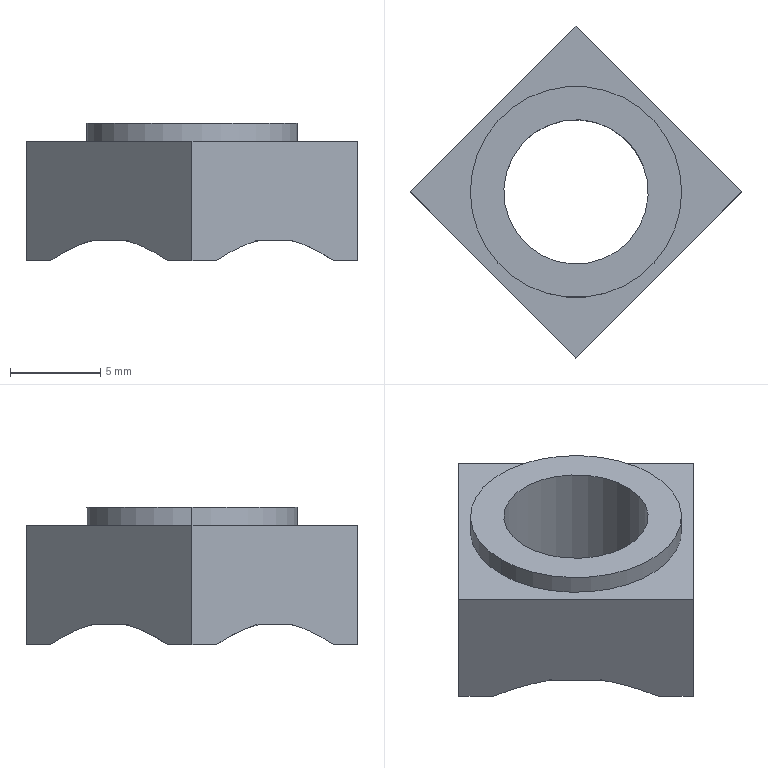Part | STEP file | Q37108 | 1 solid | 20 faces | box 18.385 x 18.385 x 7.6 mm | volume 729.18 mm3 | plane 11 | cone 5 | cylinder 4 | commonest cylinder face diameters 8 x2 11.7 x2
STEP:
#1=CARTESIAN_POINT('',(3.672,5.52,0.));
#2=VERTEX_POINT('',#1);
#3=CARTESIAN_POINT('',(5.52,3.672,0.));
#4=VERTEX_POINT('',#3);
#5=CARTESIAN_POINT('',(4.596,4.596,0.));
#6=DIRECTION('',(0.7071,-0.7071,0.));
#7=VECTOR('',#6,1.);
#8=LINE('',#5,#7);
#9=EDGE_CURVE('',#2,#4,#8,.T.);
#10=ORIENTED_EDGE('',*,*,#9,.T.);
#11=CARTESIAN_POINT('',(5.818,3.179,0.));
#12=VERTEX_POINT('',#11);
#13=CARTESIAN_POINT('',(0.,0.,0.));
#14=DIRECTION('',(0.,0.,1.));
#15=AXIS2_PLACEMENT_3D('',#13,#14,$);
#16=CIRCLE('',#15,6.63);
#17=EDGE_CURVE('',#12,#4,#16,.T.);
#18=ORIENTED_EDGE('',*,*,#17,.F.);
#19=CARTESIAN_POINT('',(5.52,-3.672,0.));
#20=VERTEX_POINT('',#19);
#21=CARTESIAN_POINT('',(0.,0.,0.));
#22=DIRECTION('',(0.,0.,1.));
#23=AXIS2_PLACEMENT_3D('',#21,#22,$);
#24=CIRCLE('',#23,6.63);
#25=EDGE_CURVE('',#20,#12,#24,.T.);
#26=ORIENTED_EDGE('',*,*,#25,.F.);
#27=CARTESIAN_POINT('',(3.672,-5.52,0.));
#28=VERTEX_POINT('',#27);
#29=CARTESIAN_POINT('',(4.596,-4.596,0.));
#30=DIRECTION('',(-0.7071,-0.7071,0.));
#31=VECTOR('',#30,1.);
#32=LINE('',#29,#31);
#33=EDGE_CURVE('',#20,#28,#32,.T.);
#34=ORIENTED_EDGE('',*,*,#33,.T.);
#35=CARTESIAN_POINT('',(-3.672,-5.52,0.));
#36=VERTEX_POINT('',#35);
#37=CARTESIAN_POINT('',(0.,0.,0.));
#38=DIRECTION('',(0.,0.,1.));
#39=AXIS2_PLACEMENT_3D('',#37,#38,$);
#40=CIRCLE('',#39,6.63);
#41=EDGE_CURVE('',#36,#28,#40,.T.);
#42=ORIENTED_EDGE('',*,*,#41,.F.);
#43=CARTESIAN_POINT('',(-5.52,-3.672,0.));
#44=VERTEX_POINT('',#43);
#45=CARTESIAN_POINT('',(-4.596,-4.596,0.));
#46=DIRECTION('',(0.7071,-0.7071,0.));
#47=VECTOR('',#46,1.);
#48=LINE('',#45,#47);
#49=EDGE_CURVE('',#44,#36,#48,.T.);
#50=ORIENTED_EDGE('',*,*,#49,.F.);
#51=CARTESIAN_POINT('',(-5.818,-3.179,0.));
#52=VERTEX_POINT('',#51);
#53=CARTESIAN_POINT('',(0.,0.,0.));
#54=DIRECTION('',(0.,0.,1.));
#55=AXIS2_PLACEMENT_3D('',#53,#54,$);
#56=CIRCLE('',#55,6.63);
#57=EDGE_CURVE('',#52,#44,#56,.T.);
#58=ORIENTED_EDGE('',*,*,#57,.F.);
#59=CARTESIAN_POINT('',(-5.52,3.672,0.));
#60=VERTEX_POINT('',#59);
#61=CARTESIAN_POINT('',(0.,0.,0.));
#62=DIRECTION('',(0.,0.,1.));
#63=AXIS2_PLACEMENT_3D('',#61,#62,$);
#64=CIRCLE('',#63,6.63);
#65=EDGE_CURVE('',#60,#52,#64,.T.);
#66=ORIENTED_EDGE('',*,*,#65,.F.);
#67=CARTESIAN_POINT('',(-3.672,5.52,0.));
#68=VERTEX_POINT('',#67);
#69=CARTESIAN_POINT('',(-4.596,4.596,0.));
#70=DIRECTION('',(0.7071,0.7071,0.));
#71=VECTOR('',#70,1.);
#72=LINE('',#69,#71);
#73=EDGE_CURVE('',#60,#68,#72,.T.);
#74=ORIENTED_EDGE('',*,*,#73,.T.);
#75=CARTESIAN_POINT('',(0.,0.,0.));
#76=DIRECTION('',(0.,0.,1.));
#77=AXIS2_PLACEMENT_3D('',#75,#76,$);
#78=CIRCLE('',#77,6.63);
#79=EDGE_CURVE('',#2,#68,#78,.T.);
#80=ORIENTED_EDGE('',*,*,#79,.F.);
#81=EDGE_LOOP('',(#10,#18,#26,#34,#42,#50,#58,#66,#74,#80));
#82=FACE_OUTER_BOUND('',#81,.T.);
#83=CARTESIAN_POINT('',(-3.51,1.918,0.));
#84=VERTEX_POINT('',#83);
#85=CARTESIAN_POINT('',(3.51,-1.918,0.));
#86=VERTEX_POINT('',#85);
#87=CARTESIAN_POINT('',(0.,0.,0.));
#88=DIRECTION('',(0.,0.,1.));
#89=AXIS2_PLACEMENT_3D('',#87,#88,$);
#90=CIRCLE('',#89,4.);
#91=EDGE_CURVE('',#84,#86,#90,.T.);
#92=ORIENTED_EDGE('',*,*,#91,.T.);
#93=CARTESIAN_POINT('',(0.,0.,0.));
#94=DIRECTION('',(0.,0.,1.));
#95=AXIS2_PLACEMENT_3D('',#93,#94,$);
#96=CIRCLE('',#95,4.);
#97=EDGE_CURVE('',#86,#84,#96,.T.);
#98=ORIENTED_EDGE('',*,*,#97,.T.);
#99=EDGE_LOOP('',(#92,#98));
#100=FACE_BOUND('',#99,.T.);
#101=CARTESIAN_POINT('',(0.,0.,0.));
#102=DIRECTION('',(0.,0.,1.));
#103=DIRECTION('',(1.,0.,0.));
#104=AXIS2_PLACEMENT_3D('',#101,#102,#103);
#105=PLANE('',#104);
#106=ADVANCED_FACE('',(#82,#100),#105,.F.);
#107=CARTESIAN_POINT('',(-1.371,7.822,-1.1));
#108=VERTEX_POINT('',#107);
#109=CARTESIAN_POINT('',(-3.672,5.52,0.));
#110=CARTESIAN_POINT('',(-3.177,6.016,-0.1159));
#111=CARTESIAN_POINT('',(-2.653,6.539,-0.3192));
#112=CARTESIAN_POINT('',(-2.077,7.115,-0.6183));
#113=CARTESIAN_POINT('',(-1.371,7.822,-1.1));
#114=B_SPLINE_CURVE_WITH_KNOTS('',4,(#109,#110,#111,#112,#113),.UNSPECIFIED.,.F.,.U.,(5,5),(0.,41.553),.UNSPECIFIED.);
#115=EDGE_CURVE('',#68,#108,#114,.T.);
#116=ORIENTED_EDGE('',*,*,#115,.T.);
#117=CARTESIAN_POINT('',(1.371,7.822,-1.1));
#118=VERTEX_POINT('',#117);
#119=CARTESIAN_POINT('',(0.,0.,-1.1));
#120=DIRECTION('',(0.,0.,-1.));
#121=AXIS2_PLACEMENT_3D('',#119,#120,$);
#122=CIRCLE('',#121,7.941);
#123=EDGE_CURVE('',#118,#108,#122,.F.);
#124=ORIENTED_EDGE('',*,*,#123,.F.);
#125=CARTESIAN_POINT('',(3.672,5.52,0.));
#126=CARTESIAN_POINT('',(3.177,6.016,-0.1159));
#127=CARTESIAN_POINT('',(2.653,6.539,-0.3192));
#128=CARTESIAN_POINT('',(2.077,7.115,-0.6183));
#129=CARTESIAN_POINT('',(1.371,7.822,-1.1));
#130=B_SPLINE_CURVE_WITH_KNOTS('',4,(#125,#126,#127,#128,#129),.UNSPECIFIED.,.F.,.U.,(5,5),(0.,41.553),.UNSPECIFIED.);
#131=EDGE_CURVE('',#2,#118,#130,.T.);
#132=ORIENTED_EDGE('',*,*,#131,.F.);
#133=ORIENTED_EDGE('',*,*,#79,.T.);
#134=EDGE_LOOP('',(#116,#124,#132,#133));
#135=FACE_OUTER_BOUND('',#134,.T.);
#136=CARTESIAN_POINT('',(0.,0.,0.));
#137=DIRECTION('',(0.,0.,-1.));
#138=DIRECTION('',(0.8776,0.4794,0.));
#139=AXIS2_PLACEMENT_3D('',#136,#137,#138);
#140=CONICAL_SURFACE('',#139,6.63,0.8727);
#141=ADVANCED_FACE('',(#135),#140,.F.);
#142=ORIENTED_EDGE('',*,*,#115,.F.);
#143=ORIENTED_EDGE('',*,*,#73,.F.);
#144=CARTESIAN_POINT('',(-7.822,1.371,-1.1));
#145=VERTEX_POINT('',#144);
#146=CARTESIAN_POINT('',(-5.52,3.672,0.));
#147=CARTESIAN_POINT('',(-5.821,3.371,-0.0704));
#148=CARTESIAN_POINT('',(-6.132,3.061,-0.1706));
#149=CARTESIAN_POINT('',(-6.456,2.736,-0.3034));
#150=CARTESIAN_POINT('',(-6.913,2.279,-0.5286));
#151=CARTESIAN_POINT('',(-7.427,1.765,-0.8406));
#152=CARTESIAN_POINT('',(-7.554,1.638,-0.921));
#153=CARTESIAN_POINT('',(-7.686,1.507,-1.007));
#154=CARTESIAN_POINT('',(-7.822,1.371,-1.1));
#155=B_SPLINE_CURVE_WITH_KNOTS('',5,(#146,#147,#148,#149,#150,#151,#152,#153,#154),.UNSPECIFIED.,.F.,.U.,(6,3,6),(0.,31.556,41.553),.UNSPECIFIED.);
#156=EDGE_CURVE('',#60,#145,#155,.T.);
#157=ORIENTED_EDGE('',*,*,#156,.T.);
#158=CARTESIAN_POINT('',(-9.192,0.,-1.1));
#159=VERTEX_POINT('',#158);
#160=CARTESIAN_POINT('',(-8.507,0.6853,-1.1));
#161=DIRECTION('',(0.7071,0.7071,0.));
#162=VECTOR('',#161,1.);
#163=LINE('',#160,#162);
#164=EDGE_CURVE('',#145,#159,#163,.F.);
#165=ORIENTED_EDGE('',*,*,#164,.T.);
#166=CARTESIAN_POINT('',(-9.192,0.,5.5));
#167=VERTEX_POINT('',#166);
#168=CARTESIAN_POINT('',(-9.192,0.,2.2));
#169=DIRECTION('',(0.,0.,1.));
#170=VECTOR('',#169,1.);
#171=LINE('',#168,#170);
#172=EDGE_CURVE('',#159,#167,#171,.T.);
#173=ORIENTED_EDGE('',*,*,#172,.T.);
#174=CARTESIAN_POINT('',(0.,9.192,5.5));
#175=VERTEX_POINT('',#174);
#176=CARTESIAN_POINT('',(-4.596,4.596,5.5));
#177=DIRECTION('',(0.7071,0.7071,0.));
#178=VECTOR('',#177,1.);
#179=LINE('',#176,#178);
#180=EDGE_CURVE('',#175,#167,#179,.F.);
#181=ORIENTED_EDGE('',*,*,#180,.F.);
#182=CARTESIAN_POINT('',(0.,9.192,-1.1));
#183=VERTEX_POINT('',#182);
#184=CARTESIAN_POINT('',(0.,9.192,2.2));
#185=DIRECTION('',(0.,0.,1.));
#186=VECTOR('',#185,1.);
#187=LINE('',#184,#186);
#188=EDGE_CURVE('',#183,#175,#187,.T.);
#189=ORIENTED_EDGE('',*,*,#188,.F.);
#190=CARTESIAN_POINT('',(-0.6853,8.507,-1.1));
#191=DIRECTION('',(0.7071,0.7071,0.));
#192=VECTOR('',#191,1.);
#193=LINE('',#190,#192);
#194=EDGE_CURVE('',#183,#108,#193,.F.);
#195=ORIENTED_EDGE('',*,*,#194,.T.);
#196=EDGE_LOOP('',(#142,#143,#157,#165,#173,#181,#189,#195));
#197=FACE_OUTER_BOUND('',#196,.T.);
#198=CARTESIAN_POINT('',(-9.192,0.,0.));
#199=DIRECTION('',(0.7071,-0.7071,0.));
#200=DIRECTION('',(0.7071,0.7071,0.));
#201=AXIS2_PLACEMENT_3D('',#198,#199,#200);
#202=PLANE('',#201);
#203=ADVANCED_FACE('',(#197),#202,.F.);
#204=CARTESIAN_POINT('',(-5.945,-3.248,-0.1208));
#205=VERTEX_POINT('',#204);
#206=CARTESIAN_POINT('',(-5.52,-3.672,0.));
#207=CARTESIAN_POINT('',(-5.659,-3.534,-0.03245));
#208=CARTESIAN_POINT('',(-5.8,-3.392,-0.07246));
#209=CARTESIAN_POINT('',(-5.945,-3.248,-0.1208));
#210=B_SPLINE_CURVE_WITH_KNOTS('',3,(#206,#207,#208,#209),.UNSPECIFIED.,.F.,.U.,(4,4),(0.,8.728),.UNSPECIFIED.);
#211=EDGE_CURVE('',#44,#205,#210,.T.);
#212=ORIENTED_EDGE('',*,*,#211,.T.);
#213=CARTESIAN_POINT('',(-7.822,-1.371,-1.1));
#214=VERTEX_POINT('',#213);
#215=CARTESIAN_POINT('',(-5.945,-3.248,-0.1208));
#216=CARTESIAN_POINT('',(-6.353,-2.839,-0.2573));
#217=CARTESIAN_POINT('',(-6.788,-2.405,-0.4537));
#218=CARTESIAN_POINT('',(-7.263,-1.929,-0.7194));
#219=CARTESIAN_POINT('',(-7.822,-1.371,-1.1));
#220=B_SPLINE_CURVE_WITH_KNOTS('',4,(#215,#216,#217,#218,#219),.UNSPECIFIED.,.F.,.U.,(5,5),(0.,32.828),.UNSPECIFIED.);
#221=EDGE_CURVE('',#205,#214,#220,.T.);
#222=ORIENTED_EDGE('',*,*,#221,.T.);
#223=CARTESIAN_POINT('',(0.,0.,-1.1));
#224=DIRECTION('',(0.,0.,-1.));
#225=AXIS2_PLACEMENT_3D('',#223,#224,$);
#226=CIRCLE('',#225,7.941);
#227=EDGE_CURVE('',#145,#214,#226,.F.);
#228=ORIENTED_EDGE('',*,*,#227,.F.);
#229=ORIENTED_EDGE('',*,*,#156,.F.);
#230=ORIENTED_EDGE('',*,*,#65,.T.);
#231=ORIENTED_EDGE('',*,*,#57,.T.);
#232=EDGE_LOOP('',(#212,#222,#228,#229,#230,#231));
#233=FACE_OUTER_BOUND('',#232,.T.);
#234=ADVANCED_FACE('',(#233),#140,.F.);
#235=ORIENTED_EDGE('',*,*,#221,.F.);
#236=ORIENTED_EDGE('',*,*,#211,.F.);
#237=ORIENTED_EDGE('',*,*,#49,.T.);
#238=CARTESIAN_POINT('',(-1.371,-7.822,-1.1));
#239=VERTEX_POINT('',#238);
#240=CARTESIAN_POINT('',(-3.672,-5.52,0.));
#241=CARTESIAN_POINT('',(-3.371,-5.821,-0.0704));
#242=CARTESIAN_POINT('',(-3.061,-6.132,-0.1706));
#243=CARTESIAN_POINT('',(-2.736,-6.456,-0.3034));
#244=CARTESIAN_POINT('',(-2.279,-6.913,-0.5286));
#245=CARTESIAN_POINT('',(-1.765,-7.427,-0.8406));
#246=CARTESIAN_POINT('',(-1.638,-7.554,-0.921));
#247=CARTESIAN_POINT('',(-1.507,-7.686,-1.007));
#248=CARTESIAN_POINT('',(-1.371,-7.822,-1.1));
#249=B_SPLINE_CURVE_WITH_KNOTS('',5,(#240,#241,#242,#243,#244,#245,#246,#247,#248),.UNSPECIFIED.,.F.,.U.,(6,3,6),(0.,31.556,41.553),.UNSPECIFIED.);
#250=EDGE_CURVE('',#36,#239,#249,.T.);
#251=ORIENTED_EDGE('',*,*,#250,.T.);
#252=CARTESIAN_POINT('',(0.,-9.192,-1.1));
#253=VERTEX_POINT('',#252);
#254=CARTESIAN_POINT('',(-0.6853,-8.507,-1.1));
#255=DIRECTION('',(-0.7071,0.7071,0.));
#256=VECTOR('',#255,1.);
#257=LINE('',#254,#256);
#258=EDGE_CURVE('',#239,#253,#257,.F.);
#259=ORIENTED_EDGE('',*,*,#258,.T.);
#260=CARTESIAN_POINT('',(0.,-9.192,5.5));
#261=VERTEX_POINT('',#260);
#262=CARTESIAN_POINT('',(0.,-9.192,2.2));
#263=DIRECTION('',(0.,0.,1.));
#264=VECTOR('',#263,1.);
#265=LINE('',#262,#264);
#266=EDGE_CURVE('',#253,#261,#265,.T.);
#267=ORIENTED_EDGE('',*,*,#266,.T.);
#268=CARTESIAN_POINT('',(-4.596,-4.596,5.5));
#269=DIRECTION('',(-0.7071,0.7071,0.));
#270=VECTOR('',#269,1.);
#271=LINE('',#268,#270);
#272=EDGE_CURVE('',#167,#261,#271,.F.);
#273=ORIENTED_EDGE('',*,*,#272,.F.);
#274=ORIENTED_EDGE('',*,*,#172,.F.);
#275=CARTESIAN_POINT('',(-8.507,-0.6853,-1.1));
#276=DIRECTION('',(-0.7071,0.7071,0.));
#277=VECTOR('',#276,1.);
#278=LINE('',#275,#277);
#279=EDGE_CURVE('',#159,#214,#278,.F.);
#280=ORIENTED_EDGE('',*,*,#279,.T.);
#281=EDGE_LOOP('',(#235,#236,#237,#251,#259,#267,#273,#274,#280));
#282=FACE_OUTER_BOUND('',#281,.T.);
#283=CARTESIAN_POINT('',(0.,-9.192,0.));
#284=DIRECTION('',(0.7071,0.7071,0.));
#285=DIRECTION('',(-0.7071,0.7071,0.));
#286=AXIS2_PLACEMENT_3D('',#283,#284,#285);
#287=PLANE('',#286);
#288=ADVANCED_FACE('',(#282),#287,.F.);
#289=CARTESIAN_POINT('',(1.371,-7.822,-1.1));
#290=VERTEX_POINT('',#289);
#291=CARTESIAN_POINT('',(3.672,-5.52,0.));
#292=CARTESIAN_POINT('',(3.177,-6.016,-0.1159));
#293=CARTESIAN_POINT('',(2.653,-6.539,-0.3192));
#294=CARTESIAN_POINT('',(2.077,-7.115,-0.6183));
#295=CARTESIAN_POINT('',(1.371,-7.822,-1.1));
#296=B_SPLINE_CURVE_WITH_KNOTS('',4,(#291,#292,#293,#294,#295),.UNSPECIFIED.,.F.,.U.,(5,5),(0.,41.553),.UNSPECIFIED.);
#297=EDGE_CURVE('',#28,#290,#296,.T.);
#298=ORIENTED_EDGE('',*,*,#297,.T.);
#299=CARTESIAN_POINT('',(0.,0.,-1.1));
#300=DIRECTION('',(0.,0.,-1.));
#301=AXIS2_PLACEMENT_3D('',#299,#300,$);
#302=CIRCLE('',#301,7.941);
#303=EDGE_CURVE('',#239,#290,#302,.F.);
#304=ORIENTED_EDGE('',*,*,#303,.F.);
#305=ORIENTED_EDGE('',*,*,#250,.F.);
#306=ORIENTED_EDGE('',*,*,#41,.T.);
#307=EDGE_LOOP('',(#298,#304,#305,#306));
#308=FACE_OUTER_BOUND('',#307,.T.);
#309=ADVANCED_FACE('',(#308),#140,.F.);
#310=ORIENTED_EDGE('',*,*,#297,.F.);
#311=ORIENTED_EDGE('',*,*,#33,.F.);
#312=CARTESIAN_POINT('',(7.822,-1.371,-1.1));
#313=VERTEX_POINT('',#312);
#314=CARTESIAN_POINT('',(5.52,-3.672,0.));
#315=CARTESIAN_POINT('',(5.821,-3.371,-0.0704));
#316=CARTESIAN_POINT('',(6.132,-3.061,-0.1706));
#317=CARTESIAN_POINT('',(6.456,-2.736,-0.3034));
#318=CARTESIAN_POINT('',(6.913,-2.279,-0.5286));
#319=CARTESIAN_POINT('',(7.427,-1.765,-0.8406));
#320=CARTESIAN_POINT('',(7.554,-1.638,-0.921));
#321=CARTESIAN_POINT('',(7.686,-1.507,-1.007));
#322=CARTESIAN_POINT('',(7.822,-1.371,-1.1));
#323=B_SPLINE_CURVE_WITH_KNOTS('',5,(#314,#315,#316,#317,#318,#319,#320,#321,#322),.UNSPECIFIED.,.F.,.U.,(6,3,6),(0.,31.556,41.553),.UNSPECIFIED.);
#324=EDGE_CURVE('',#20,#313,#323,.T.);
#325=ORIENTED_EDGE('',*,*,#324,.T.);
#326=CARTESIAN_POINT('',(9.192,0.,-1.1));
#327=VERTEX_POINT('',#326);
#328=CARTESIAN_POINT('',(8.507,-0.6853,-1.1));
#329=DIRECTION('',(-0.7071,-0.7071,0.));
#330=VECTOR('',#329,1.);
#331=LINE('',#328,#330);
#332=EDGE_CURVE('',#313,#327,#331,.F.);
#333=ORIENTED_EDGE('',*,*,#332,.T.);
#334=CARTESIAN_POINT('',(9.192,0.,5.5));
#335=VERTEX_POINT('',#334);
#336=CARTESIAN_POINT('',(9.192,0.,2.2));
#337=DIRECTION('',(0.,0.,1.));
#338=VECTOR('',#337,1.);
#339=LINE('',#336,#338);
#340=EDGE_CURVE('',#327,#335,#339,.T.);
#341=ORIENTED_EDGE('',*,*,#340,.T.);
#342=CARTESIAN_POINT('',(4.596,-4.596,5.5));
#343=DIRECTION('',(-0.7071,-0.7071,0.));
#344=VECTOR('',#343,1.);
#345=LINE('',#342,#344);
#346=EDGE_CURVE('',#261,#335,#345,.F.);
#347=ORIENTED_EDGE('',*,*,#346,.F.);
#348=ORIENTED_EDGE('',*,*,#266,.F.);
#349=CARTESIAN_POINT('',(0.6853,-8.507,-1.1));
#350=DIRECTION('',(-0.7071,-0.7071,0.));
#351=VECTOR('',#350,1.);
#352=LINE('',#349,#351);
#353=EDGE_CURVE('',#253,#290,#352,.F.);
#354=ORIENTED_EDGE('',*,*,#353,.T.);
#355=EDGE_LOOP('',(#310,#311,#325,#333,#341,#347,#348,#354));
#356=FACE_OUTER_BOUND('',#355,.T.);
#357=CARTESIAN_POINT('',(9.192,0.,0.));
#358=DIRECTION('',(-0.7071,0.7071,0.));
#359=DIRECTION('',(-0.7071,-0.7071,0.));
#360=AXIS2_PLACEMENT_3D('',#357,#358,#359);
#361=PLANE('',#360);
#362=ADVANCED_FACE('',(#356),#361,.F.);
#363=CARTESIAN_POINT('',(5.945,3.248,-0.1208));
#364=VERTEX_POINT('',#363);
#365=CARTESIAN_POINT('',(7.822,1.371,-1.1));
#366=VERTEX_POINT('',#365);
#367=CARTESIAN_POINT('',(5.945,3.248,-0.1208));
#368=CARTESIAN_POINT('',(6.353,2.839,-0.2573));
#369=CARTESIAN_POINT('',(6.788,2.405,-0.4537));
#370=CARTESIAN_POINT('',(7.263,1.929,-0.7194));
#371=CARTESIAN_POINT('',(7.822,1.371,-1.1));
#372=B_SPLINE_CURVE_WITH_KNOTS('',4,(#367,#368,#369,#370,#371),.UNSPECIFIED.,.F.,.U.,(5,5),(0.,32.828),.UNSPECIFIED.);
#373=EDGE_CURVE('',#364,#366,#372,.T.);
#374=ORIENTED_EDGE('',*,*,#373,.T.);
#375=CARTESIAN_POINT('',(0.,0.,-1.1));
#376=DIRECTION('',(0.,0.,-1.));
#377=AXIS2_PLACEMENT_3D('',#375,#376,$);
#378=CIRCLE('',#377,7.941);
#379=EDGE_CURVE('',#313,#366,#378,.F.);
#380=ORIENTED_EDGE('',*,*,#379,.F.);
#381=ORIENTED_EDGE('',*,*,#324,.F.);
#382=ORIENTED_EDGE('',*,*,#25,.T.);
#383=CARTESIAN_POINT('',(6.461,3.53,-0.6143));
#384=DIRECTION('',(0.6723,0.3673,-0.6428));
#385=VECTOR('',#384,1.);
#386=LINE('',#383,#385);
#387=EDGE_CURVE('',#12,#364,#386,.T.);
#388=ORIENTED_EDGE('',*,*,#387,.T.);
#389=EDGE_LOOP('',(#374,#380,#381,#382,#388));
#390=FACE_OUTER_BOUND('',#389,.T.);
#391=ADVANCED_FACE('',(#390),#140,.F.);
#392=CARTESIAN_POINT('',(5.52,3.672,0.));
#393=CARTESIAN_POINT('',(5.659,3.534,-0.03245));
#394=CARTESIAN_POINT('',(5.8,3.392,-0.07246));
#395=CARTESIAN_POINT('',(5.945,3.248,-0.1208));
#396=B_SPLINE_CURVE_WITH_KNOTS('',3,(#392,#393,#394,#395),.UNSPECIFIED.,.F.,.U.,(4,4),(0.,8.728),.UNSPECIFIED.);
#397=EDGE_CURVE('',#4,#364,#396,.T.);
#398=ORIENTED_EDGE('',*,*,#397,.T.);
#399=ORIENTED_EDGE('',*,*,#387,.F.);
#400=ORIENTED_EDGE('',*,*,#17,.T.);
#401=EDGE_LOOP('',(#398,#399,#400));
#402=FACE_OUTER_BOUND('',#401,.T.);
#403=ADVANCED_FACE('',(#402),#140,.F.);
#404=ORIENTED_EDGE('',*,*,#373,.F.);
#405=ORIENTED_EDGE('',*,*,#397,.F.);
#406=ORIENTED_EDGE('',*,*,#9,.F.);
#407=ORIENTED_EDGE('',*,*,#131,.T.);
#408=CARTESIAN_POINT('',(0.6853,8.507,-1.1));
#409=DIRECTION('',(0.7071,-0.7071,0.));
#410=VECTOR('',#409,1.);
#411=LINE('',#408,#410);
#412=EDGE_CURVE('',#118,#183,#411,.F.);
#413=ORIENTED_EDGE('',*,*,#412,.T.);
#414=ORIENTED_EDGE('',*,*,#188,.T.);
#415=CARTESIAN_POINT('',(4.596,4.596,5.5));
#416=DIRECTION('',(0.7071,-0.7071,0.));
#417=VECTOR('',#416,1.);
#418=LINE('',#415,#417);
#419=EDGE_CURVE('',#335,#175,#418,.F.);
#420=ORIENTED_EDGE('',*,*,#419,.F.);
#421=ORIENTED_EDGE('',*,*,#340,.F.);
#422=CARTESIAN_POINT('',(8.507,0.6853,-1.1));
#423=DIRECTION('',(0.7071,-0.7071,0.));
#424=VECTOR('',#423,1.);
#425=LINE('',#422,#424);
#426=EDGE_CURVE('',#327,#366,#425,.F.);
#427=ORIENTED_EDGE('',*,*,#426,.T.);
#428=EDGE_LOOP('',(#404,#405,#406,#407,#413,#414,#420,#421,#427));
#429=FACE_OUTER_BOUND('',#428,.T.);
#430=CARTESIAN_POINT('',(0.,9.192,0.));
#431=DIRECTION('',(-0.7071,-0.7071,0.));
#432=DIRECTION('',(0.7071,-0.7071,0.));
#433=AXIS2_PLACEMENT_3D('',#430,#431,#432);
#434=PLANE('',#433);
#435=ADVANCED_FACE('',(#429),#434,.F.);
#436=ORIENTED_EDGE('',*,*,#97,.F.);
#437=CARTESIAN_POINT('',(3.51,-1.918,6.5));
#438=VERTEX_POINT('',#437);
#439=CARTESIAN_POINT('',(3.51,-1.918,2.7));
#440=DIRECTION('',(0.,0.,-1.));
#441=VECTOR('',#440,1.);
#442=LINE('',#439,#441);
#443=EDGE_CURVE('',#86,#438,#442,.F.);
#444=ORIENTED_EDGE('',*,*,#443,.T.);
#445=CARTESIAN_POINT('',(-3.51,1.918,6.5));
#446=VERTEX_POINT('',#445);
#447=CARTESIAN_POINT('',(0.,0.,6.5));
#448=DIRECTION('',(0.,0.,-1.));
#449=AXIS2_PLACEMENT_3D('',#447,#448,$);
#450=CIRCLE('',#449,4.);
#451=EDGE_CURVE('',#438,#446,#450,.F.);
#452=ORIENTED_EDGE('',*,*,#451,.T.);
#453=CARTESIAN_POINT('',(-3.51,1.918,2.7));
#454=DIRECTION('',(0.,0.,-1.));
#455=VECTOR('',#454,1.);
#456=LINE('',#453,#455);
#457=EDGE_CURVE('',#84,#446,#456,.F.);
#458=ORIENTED_EDGE('',*,*,#457,.F.);
#459=EDGE_LOOP('',(#436,#444,#452,#458));
#460=FACE_OUTER_BOUND('',#459,.T.);
#461=CARTESIAN_POINT('',(0.,0.,6.2));
#462=DIRECTION('',(0.,0.,-1.));
#463=DIRECTION('',(0.8776,-0.4794,0.));
#464=AXIS2_PLACEMENT_3D('',#461,#462,#463);
#465=CYLINDRICAL_SURFACE('',#464,4.);
#466=ADVANCED_FACE('',(#460),#465,.F.);
#467=ORIENTED_EDGE('',*,*,#91,.F.);
#468=ORIENTED_EDGE('',*,*,#457,.T.);
#469=CARTESIAN_POINT('',(0.,0.,6.5));
#470=DIRECTION('',(0.,0.,-1.));
#471=AXIS2_PLACEMENT_3D('',#469,#470,$);
#472=CIRCLE('',#471,4.);
#473=EDGE_CURVE('',#446,#438,#472,.F.);
#474=ORIENTED_EDGE('',*,*,#473,.T.);
#475=ORIENTED_EDGE('',*,*,#443,.F.);
#476=EDGE_LOOP('',(#467,#468,#474,#475));
#477=FACE_OUTER_BOUND('',#476,.T.);
#478=ADVANCED_FACE('',(#477),#465,.F.);
#479=ORIENTED_EDGE('',*,*,#123,.T.);
#480=ORIENTED_EDGE('',*,*,#194,.F.);
#481=ORIENTED_EDGE('',*,*,#412,.F.);
#482=EDGE_LOOP('',(#479,#480,#481));
#483=FACE_OUTER_BOUND('',#482,.T.);
#484=CARTESIAN_POINT('',(0.,0.,-1.1));
#485=DIRECTION('',(0.,0.,1.));
#486=DIRECTION('',(1.,0.,0.));
#487=AXIS2_PLACEMENT_3D('',#484,#485,#486);
#488=PLANE('',#487);
#489=ADVANCED_FACE('',(#483),#488,.F.);
#490=ORIENTED_EDGE('',*,*,#227,.T.);
#491=ORIENTED_EDGE('',*,*,#279,.F.);
#492=ORIENTED_EDGE('',*,*,#164,.F.);
#493=EDGE_LOOP('',(#490,#491,#492));
#494=FACE_OUTER_BOUND('',#493,.T.);
#495=ADVANCED_FACE('',(#494),#488,.F.);
#496=ORIENTED_EDGE('',*,*,#272,.T.);
#497=ORIENTED_EDGE('',*,*,#346,.T.);
#498=ORIENTED_EDGE('',*,*,#419,.T.);
#499=ORIENTED_EDGE('',*,*,#180,.T.);
#500=EDGE_LOOP('',(#496,#497,#498,#499));
#501=FACE_OUTER_BOUND('',#500,.T.);
#502=CARTESIAN_POINT('',(5.85,0.,5.5));
#503=VERTEX_POINT('',#502);
#504=CARTESIAN_POINT('',(-5.85,0.,5.5));
#505=VERTEX_POINT('',#504);
#506=CARTESIAN_POINT('',(0.,0.,5.5));
#507=DIRECTION('',(0.,0.,1.));
#508=AXIS2_PLACEMENT_3D('',#506,#507,$);
#509=CIRCLE('',#508,5.85);
#510=EDGE_CURVE('',#503,#505,#509,.T.);
#511=ORIENTED_EDGE('',*,*,#510,.F.);
#512=CARTESIAN_POINT('',(0.,0.,5.5));
#513=DIRECTION('',(0.,0.,1.));
#514=AXIS2_PLACEMENT_3D('',#512,#513,$);
#515=CIRCLE('',#514,5.85);
#516=EDGE_CURVE('',#505,#503,#515,.T.);
#517=ORIENTED_EDGE('',*,*,#516,.F.);
#518=EDGE_LOOP('',(#511,#517));
#519=FACE_BOUND('',#518,.T.);
#520=CARTESIAN_POINT('',(0.,0.,5.5));
#521=DIRECTION('',(0.,0.,1.));
#522=DIRECTION('',(1.,0.,0.));
#523=AXIS2_PLACEMENT_3D('',#520,#521,#522);
#524=PLANE('',#523);
#525=ADVANCED_FACE('',(#501,#519),#524,.T.);
#526=ORIENTED_EDGE('',*,*,#303,.T.);
#527=ORIENTED_EDGE('',*,*,#353,.F.);
#528=ORIENTED_EDGE('',*,*,#258,.F.);
#529=EDGE_LOOP('',(#526,#527,#528));
#530=FACE_OUTER_BOUND('',#529,.T.);
#531=ADVANCED_FACE('',(#530),#488,.F.);
#532=ORIENTED_EDGE('',*,*,#379,.T.);
#533=ORIENTED_EDGE('',*,*,#426,.F.);
#534=ORIENTED_EDGE('',*,*,#332,.F.);
#535=EDGE_LOOP('',(#532,#533,#534));
#536=FACE_OUTER_BOUND('',#535,.T.);
#537=ADVANCED_FACE('',(#536),#488,.F.);
#538=CARTESIAN_POINT('',(5.85,0.,6.5));
#539=VERTEX_POINT('',#538);
#540=CARTESIAN_POINT('',(-5.85,0.,6.5));
#541=VERTEX_POINT('',#540);
#542=CARTESIAN_POINT('',(0.,0.,6.5));
#543=DIRECTION('',(0.,0.,1.));
#544=AXIS2_PLACEMENT_3D('',#542,#543,$);
#545=CIRCLE('',#544,5.85);
#546=EDGE_CURVE('',#539,#541,#545,.T.);
#547=ORIENTED_EDGE('',*,*,#546,.T.);
#548=CARTESIAN_POINT('',(0.,0.,6.5));
#549=DIRECTION('',(0.,0.,1.));
#550=AXIS2_PLACEMENT_3D('',#548,#549,$);
#551=CIRCLE('',#550,5.85);
#552=EDGE_CURVE('',#541,#539,#551,.T.);
#553=ORIENTED_EDGE('',*,*,#552,.T.);
#554=EDGE_LOOP('',(#547,#553));
#555=FACE_OUTER_BOUND('',#554,.T.);
#556=ORIENTED_EDGE('',*,*,#473,.F.);
#557=ORIENTED_EDGE('',*,*,#451,.F.);
#558=EDGE_LOOP('',(#556,#557));
#559=FACE_BOUND('',#558,.T.);
#560=CARTESIAN_POINT('',(0.,0.,6.5));
#561=DIRECTION('',(0.,0.,1.));
#562=DIRECTION('',(1.,0.,0.));
#563=AXIS2_PLACEMENT_3D('',#560,#561,#562);
#564=PLANE('',#563);
#565=ADVANCED_FACE('',(#555,#559),#564,.T.);
#566=CARTESIAN_POINT('',(5.85,0.,6.));
#567=DIRECTION('',(0.,0.,1.));
#568=VECTOR('',#567,1.);
#569=LINE('',#566,#568);
#570=EDGE_CURVE('',#503,#539,#569,.T.);
#571=ORIENTED_EDGE('',*,*,#570,.F.);
#572=ORIENTED_EDGE('',*,*,#510,.T.);
#573=CARTESIAN_POINT('',(-5.85,0.,6.));
#574=DIRECTION('',(0.,0.,1.));
#575=VECTOR('',#574,1.);
#576=LINE('',#573,#575);
#577=EDGE_CURVE('',#505,#541,#576,.T.);
#578=ORIENTED_EDGE('',*,*,#577,.T.);
#579=ORIENTED_EDGE('',*,*,#546,.F.);
#580=EDGE_LOOP('',(#571,#572,#578,#579));
#581=FACE_OUTER_BOUND('',#580,.T.);
#582=CARTESIAN_POINT('',(0.,0.,6.));
#583=DIRECTION('',(0.,0.,1.));
#584=DIRECTION('',(1.,0.,0.));
#585=AXIS2_PLACEMENT_3D('',#582,#583,#584);
#586=CYLINDRICAL_SURFACE('',#585,5.85);
#587=ADVANCED_FACE('',(#581),#586,.T.);
#588=ORIENTED_EDGE('',*,*,#577,.F.);
#589=ORIENTED_EDGE('',*,*,#516,.T.);
#590=ORIENTED_EDGE('',*,*,#570,.T.);
#591=ORIENTED_EDGE('',*,*,#552,.F.);
#592=EDGE_LOOP('',(#588,#589,#590,#591));
#593=FACE_OUTER_BOUND('',#592,.T.);
#594=ADVANCED_FACE('',(#593),#586,.T.);
#595=CLOSED_SHELL('',(#106,#141,#203,#234,#288,#309,#362,#391,#403,#435,#466,#478,#489,#495,#525,#531,#537,#565,#587,#594));
#596=MANIFOLD_SOLID_BREP('',#595);
#597=(LENGTH_UNIT()NAMED_UNIT(*)SI_UNIT(.MILLI.,.METRE.));
#598=UNCERTAINTY_MEASURE_WITH_UNIT(LENGTH_MEASURE(0.005),#597,'','');
#599=(NAMED_UNIT(*)PLANE_ANGLE_UNIT()SI_UNIT($,.RADIAN.));
#600=(NAMED_UNIT(*)SI_UNIT($,.STERADIAN.)SOLID_ANGLE_UNIT());
#601=(GEOMETRIC_REPRESENTATION_CONTEXT(3)GLOBAL_UNCERTAINTY_ASSIGNED_CONTEXT((#598))GLOBAL_UNIT_ASSIGNED_CONTEXT((#597,#599,#600))REPRESENTATION_CONTEXT('',''));
#602=ADVANCED_BREP_SHAPE_REPRESENTATION('',(#596),#601);